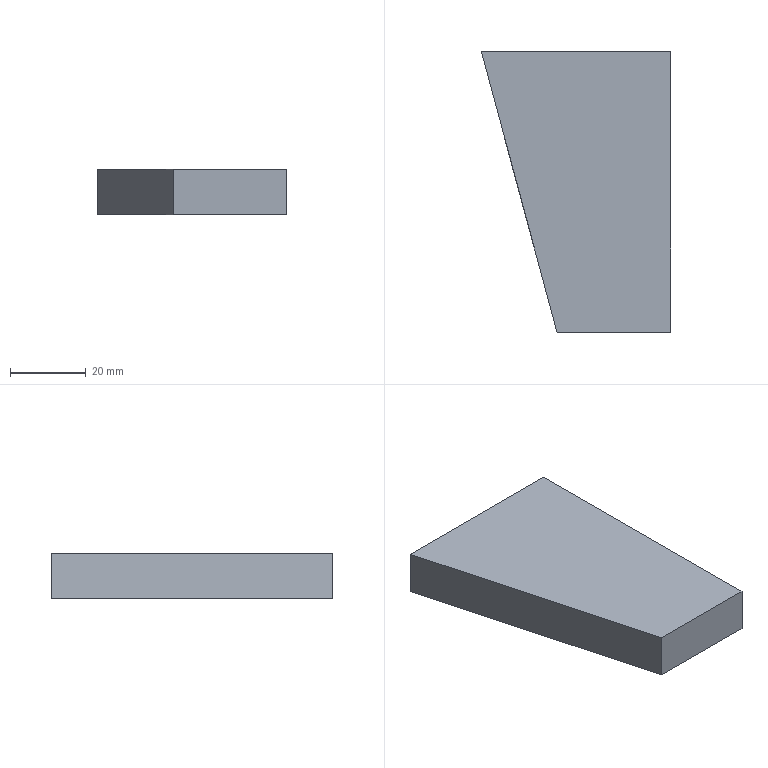Part | SolidWorks | features FlatPattern 1, SMBaseFlange 1, SheetMetal 1 | 1 solid | 6 faces | box 50 x 74 x 12 mm | volume 35520 mm3 | plane 6
STEP:
#1=CARTESIAN_POINT('',(-20.,74.,0.));
#2=VERTEX_POINT('',#1);
#3=CARTESIAN_POINT('',(0.,0.,0.));
#4=VERTEX_POINT('',#3);
#5=CARTESIAN_POINT('',(-20.,74.,0.));
#6=DIRECTION('',(0.2609,-0.9654,0.));
#7=VECTOR('',#6,1000.);
#8=LINE('',#5,#7);
#9=EDGE_CURVE('',#2,#4,#8,.T.);
#10=ORIENTED_EDGE('',*,*,#9,.F.);
#11=CARTESIAN_POINT('',(-20.,74.,-12.));
#12=VERTEX_POINT('',#11);
#13=CARTESIAN_POINT('',(-20.,74.,-12.));
#14=DIRECTION('',(0.,0.,1.));
#15=VECTOR('',#14,1000.);
#16=LINE('',#13,#15);
#17=EDGE_CURVE('',#12,#2,#16,.T.);
#18=ORIENTED_EDGE('',*,*,#17,.F.);
#19=CARTESIAN_POINT('',(0.,0.,-12.));
#20=VERTEX_POINT('',#19);
#21=CARTESIAN_POINT('',(-20.,74.,-12.));
#22=DIRECTION('',(0.2609,-0.9654,0.));
#23=VECTOR('',#22,1000.);
#24=LINE('',#21,#23);
#25=EDGE_CURVE('',#12,#20,#24,.T.);
#26=ORIENTED_EDGE('',*,*,#25,.T.);
#27=CARTESIAN_POINT('',(0.,0.,-12.));
#28=DIRECTION('',(0.,0.,1.));
#29=VECTOR('',#28,1000.);
#30=LINE('',#27,#29);
#31=EDGE_CURVE('',#20,#4,#30,.T.);
#32=ORIENTED_EDGE('',*,*,#31,.T.);
#33=EDGE_LOOP('',(#10,#18,#26,#32));
#34=FACE_OUTER_BOUND('',#33,.T.);
#35=CARTESIAN_POINT('',(-20.,74.,-12.));
#36=DIRECTION('',(-0.9654,-0.2609,0.));
#37=DIRECTION('',(0.2609,-0.9654,0.));
#38=AXIS2_PLACEMENT_3D('',#35,#36,#37);
#39=PLANE('',#38);
#40=ADVANCED_FACE('',(#34),#39,.T.);
#41=CARTESIAN_POINT('',(30.,74.,0.));
#42=VERTEX_POINT('',#41);
#43=CARTESIAN_POINT('',(-20.,74.,0.));
#44=DIRECTION('',(-1.,0.,0.));
#45=VECTOR('',#44,1000.);
#46=LINE('',#43,#45);
#47=EDGE_CURVE('',#42,#2,#46,.T.);
#48=ORIENTED_EDGE('',*,*,#47,.F.);
#49=CARTESIAN_POINT('',(30.,74.,-12.));
#50=VERTEX_POINT('',#49);
#51=CARTESIAN_POINT('',(30.,74.,-12.));
#52=DIRECTION('',(0.,0.,1.));
#53=VECTOR('',#52,1000.);
#54=LINE('',#51,#53);
#55=EDGE_CURVE('',#50,#42,#54,.T.);
#56=ORIENTED_EDGE('',*,*,#55,.F.);
#57=CARTESIAN_POINT('',(-20.,74.,-12.));
#58=DIRECTION('',(-1.,0.,0.));
#59=VECTOR('',#58,1000.);
#60=LINE('',#57,#59);
#61=EDGE_CURVE('',#50,#12,#60,.T.);
#62=ORIENTED_EDGE('',*,*,#61,.T.);
#63=ORIENTED_EDGE('',*,*,#17,.T.);
#64=EDGE_LOOP('',(#48,#56,#62,#63));
#65=FACE_OUTER_BOUND('',#64,.T.);
#66=CARTESIAN_POINT('',(-20.,74.,-12.));
#67=DIRECTION('',(0.,1.,0.));
#68=DIRECTION('',(0.,0.,1.));
#69=AXIS2_PLACEMENT_3D('',#66,#67,#68);
#70=PLANE('',#69);
#71=ADVANCED_FACE('',(#65),#70,.T.);
#72=CARTESIAN_POINT('',(30.,0.,0.));
#73=VERTEX_POINT('',#72);
#74=CARTESIAN_POINT('',(30.,0.,0.));
#75=DIRECTION('',(0.,1.,0.));
#76=VECTOR('',#75,1000.);
#77=LINE('',#74,#76);
#78=EDGE_CURVE('',#73,#42,#77,.T.);
#79=ORIENTED_EDGE('',*,*,#78,.F.);
#80=CARTESIAN_POINT('',(30.,0.,-12.));
#81=VERTEX_POINT('',#80);
#82=CARTESIAN_POINT('',(30.,0.,-12.));
#83=DIRECTION('',(0.,0.,1.));
#84=VECTOR('',#83,1000.);
#85=LINE('',#82,#84);
#86=EDGE_CURVE('',#81,#73,#85,.T.);
#87=ORIENTED_EDGE('',*,*,#86,.F.);
#88=CARTESIAN_POINT('',(30.,0.,-12.));
#89=DIRECTION('',(0.,1.,0.));
#90=VECTOR('',#89,1000.);
#91=LINE('',#88,#90);
#92=EDGE_CURVE('',#81,#50,#91,.T.);
#93=ORIENTED_EDGE('',*,*,#92,.T.);
#94=ORIENTED_EDGE('',*,*,#55,.T.);
#95=EDGE_LOOP('',(#79,#87,#93,#94));
#96=FACE_OUTER_BOUND('',#95,.T.);
#97=CARTESIAN_POINT('',(30.,0.,-12.));
#98=DIRECTION('',(1.,0.,0.));
#99=DIRECTION('',(0.,0.,-1.));
#100=AXIS2_PLACEMENT_3D('',#97,#98,#99);
#101=PLANE('',#100);
#102=ADVANCED_FACE('',(#96),#101,.T.);
#103=CARTESIAN_POINT('',(0.,0.,0.));
#104=DIRECTION('',(1.,0.,0.));
#105=VECTOR('',#104,1000.);
#106=LINE('',#103,#105);
#107=EDGE_CURVE('',#4,#73,#106,.T.);
#108=ORIENTED_EDGE('',*,*,#107,.F.);
#109=ORIENTED_EDGE('',*,*,#31,.F.);
#110=CARTESIAN_POINT('',(0.,0.,-12.));
#111=DIRECTION('',(1.,0.,0.));
#112=VECTOR('',#111,1000.);
#113=LINE('',#110,#112);
#114=EDGE_CURVE('',#20,#81,#113,.T.);
#115=ORIENTED_EDGE('',*,*,#114,.T.);
#116=ORIENTED_EDGE('',*,*,#86,.T.);
#117=EDGE_LOOP('',(#108,#109,#115,#116));
#118=FACE_OUTER_BOUND('',#117,.T.);
#119=CARTESIAN_POINT('',(0.,0.,-12.));
#120=DIRECTION('',(0.,-1.,0.));
#121=DIRECTION('',(0.,0.,-1.));
#122=AXIS2_PLACEMENT_3D('',#119,#120,#121);
#123=PLANE('',#122);
#124=ADVANCED_FACE('',(#118),#123,.T.);
#125=ORIENTED_EDGE('',*,*,#25,.F.);
#126=ORIENTED_EDGE('',*,*,#61,.F.);
#127=ORIENTED_EDGE('',*,*,#92,.F.);
#128=ORIENTED_EDGE('',*,*,#114,.F.);
#129=EDGE_LOOP('',(#125,#126,#127,#128));
#130=FACE_OUTER_BOUND('',#129,.T.);
#131=CARTESIAN_POINT('',(0.,0.,-12.));
#132=DIRECTION('',(0.,0.,1.));
#133=DIRECTION('',(1.,0.,0.));
#134=AXIS2_PLACEMENT_3D('',#131,#132,#133);
#135=PLANE('',#134);
#136=ADVANCED_FACE('',(#130),#135,.F.);
#137=ORIENTED_EDGE('',*,*,#9,.T.);
#138=ORIENTED_EDGE('',*,*,#107,.T.);
#139=ORIENTED_EDGE('',*,*,#78,.T.);
#140=ORIENTED_EDGE('',*,*,#47,.T.);
#141=EDGE_LOOP('',(#137,#138,#139,#140));
#142=FACE_OUTER_BOUND('',#141,.T.);
#143=CARTESIAN_POINT('',(0.,0.,0.));
#144=DIRECTION('',(0.,0.,1.));
#145=DIRECTION('',(1.,0.,0.));
#146=AXIS2_PLACEMENT_3D('',#143,#144,#145);
#147=PLANE('',#146);
#148=ADVANCED_FACE('',(#142),#147,.T.);
#149=CLOSED_SHELL('',(#40,#71,#102,#124,#136,#148));
#150=MANIFOLD_SOLID_BREP('',#149);
#151=CARTESIAN_POINT('',(0.,0.,0.));
#152=DIRECTION('',(0.,0.,1.));
#153=DIRECTION('',(1.,0.,0.));
#154=AXIS2_PLACEMENT_3D('',#151,#152,#153);
#155=(LENGTH_UNIT()NAMED_UNIT(*)SI_UNIT(.MILLI.,.METRE.));
#156=UNCERTAINTY_MEASURE_WITH_UNIT(LENGTH_MEASURE(0.00001),#155,'','');
#157=(NAMED_UNIT(*)PLANE_ANGLE_UNIT()SI_UNIT($,.RADIAN.));
#158=(NAMED_UNIT(*)SI_UNIT($,.STERADIAN.)SOLID_ANGLE_UNIT());
#159=(GEOMETRIC_REPRESENTATION_CONTEXT(3)GLOBAL_UNCERTAINTY_ASSIGNED_CONTEXT((#156))GLOBAL_UNIT_ASSIGNED_CONTEXT((#155,#157,#158))REPRESENTATION_CONTEXT('',''));
#160=ADVANCED_BREP_SHAPE_REPRESENTATION('',(#150,#154),#159);